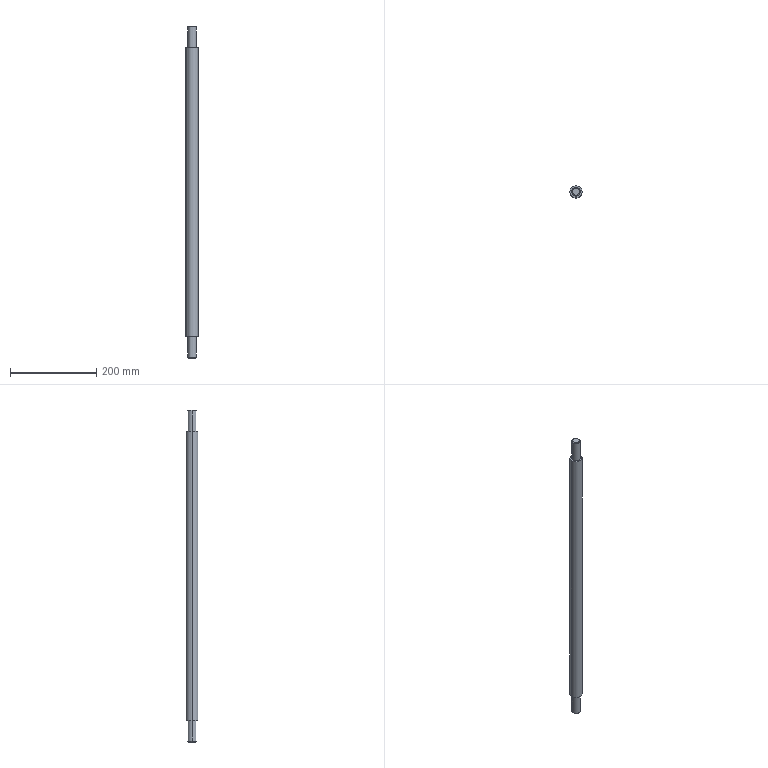Part | Creo | features DATUM PLANE 3, CURVE 2, PROTRUSION 2, CHAMFER 1, COORDINATE SYSTEM 1 | 1 solid | 14 faces | box 28 x 28 x 770 mm | volume 443735 mm3 | cylinder 6 | plane 4 | cone 4 | commonest cylinder face diameters 20 x4 28 x2
STEP:
#1=CARTESIAN_POINT('',(0.,0.,0.));
#2=DIRECTION('',(0.,0.,1.));
#3=DIRECTION('',(1.,0.,0.));
#4=AXIS2_PLACEMENT_3D('',#1,#2,#3);
#5=CARTESIAN_POINT('',(14.,0.,-335.));
#6=VERTEX_POINT('',#5);
#7=CARTESIAN_POINT('',(-14.,0.,-335.));
#8=VERTEX_POINT('',#7);
#9=CARTESIAN_POINT('',(0.,0.,-335.));
#10=DIRECTION('',(0.,0.,1.));
#11=DIRECTION('',(1.,0.,0.));
#12=AXIS2_PLACEMENT_3D('',#9,#10,#11);
#13=CIRCLE('',#12,14.);
#14=EDGE_CURVE('',#6,#8,#13,.T.);
#15=ORIENTED_EDGE('',*,*,#14,.T.);
#16=CARTESIAN_POINT('',(0.,0.,-335.));
#17=DIRECTION('',(0.,0.,1.));
#18=DIRECTION('',(-1.,0.,0.));
#19=AXIS2_PLACEMENT_3D('',#16,#17,#18);
#20=CIRCLE('',#19,14.);
#21=EDGE_CURVE('',#8,#6,#20,.T.);
#22=ORIENTED_EDGE('',*,*,#21,.T.);
#23=EDGE_LOOP('',(#15,#22));
#24=FACE_OUTER_BOUND('',#23,.F.);
#25=CARTESIAN_POINT('',(10.,0.,-335.));
#26=VERTEX_POINT('',#25);
#27=CARTESIAN_POINT('',(-10.,0.,-335.));
#28=VERTEX_POINT('',#27);
#29=CARTESIAN_POINT('',(0.,0.,-335.));
#30=DIRECTION('',(0.,0.,1.));
#31=DIRECTION('',(1.,0.,0.));
#32=AXIS2_PLACEMENT_3D('',#29,#30,#31);
#33=CIRCLE('',#32,10.);
#34=EDGE_CURVE('',#26,#28,#33,.T.);
#35=ORIENTED_EDGE('',*,*,#34,.F.);
#36=CARTESIAN_POINT('',(0.,0.,-335.));
#37=DIRECTION('',(0.,0.,1.));
#38=DIRECTION('',(-1.,0.,0.));
#39=AXIS2_PLACEMENT_3D('',#36,#37,#38);
#40=CIRCLE('',#39,10.);
#41=EDGE_CURVE('',#28,#26,#40,.T.);
#42=ORIENTED_EDGE('',*,*,#41,.F.);
#43=EDGE_LOOP('',(#35,#42));
#44=FACE_BOUND('',#43,.F.);
#45=CARTESIAN_POINT('',(0.,0.,-335.));
#46=DIRECTION('',(0.,0.,1.));
#47=DIRECTION('',(1.,0.,0.));
#48=AXIS2_PLACEMENT_3D('',#45,#46,#47);
#49=PLANE('',#48);
#50=ADVANCED_FACE('',(#24,#44),#49,.F.);
#51=ORIENTED_EDGE('',*,*,#14,.F.);
#52=CARTESIAN_POINT('',(14.,0.,335.));
#53=VERTEX_POINT('',#52);
#54=CARTESIAN_POINT('',(14.,0.,-335.));
#55=DIRECTION('',(0.,0.,1.));
#56=VECTOR('',#55,670.);
#57=LINE('',#54,#56);
#58=EDGE_CURVE('',#6,#53,#57,.T.);
#59=ORIENTED_EDGE('',*,*,#58,.T.);
#60=CARTESIAN_POINT('',(-14.,0.,335.));
#61=VERTEX_POINT('',#60);
#62=CARTESIAN_POINT('',(0.,0.,335.));
#63=DIRECTION('',(0.,0.,1.));
#64=DIRECTION('',(1.,0.,0.));
#65=AXIS2_PLACEMENT_3D('',#62,#63,#64);
#66=CIRCLE('',#65,14.);
#67=EDGE_CURVE('',#53,#61,#66,.T.);
#68=ORIENTED_EDGE('',*,*,#67,.T.);
#69=CARTESIAN_POINT('',(-14.,0.,-335.));
#70=DIRECTION('',(0.,0.,1.));
#71=VECTOR('',#70,670.);
#72=LINE('',#69,#71);
#73=EDGE_CURVE('',#8,#61,#72,.T.);
#74=ORIENTED_EDGE('',*,*,#73,.F.);
#75=EDGE_LOOP('',(#51,#59,#68,#74));
#76=FACE_OUTER_BOUND('',#75,.F.);
#77=CARTESIAN_POINT('',(0.,0.,-335.));
#78=DIRECTION('',(0.,0.,1.));
#79=DIRECTION('',(1.,0.,0.));
#80=AXIS2_PLACEMENT_3D('',#77,#78,#79);
#81=CYLINDRICAL_SURFACE('',#80,14.);
#82=ADVANCED_FACE('',(#76),#81,.T.);
#83=ORIENTED_EDGE('',*,*,#21,.F.);
#84=ORIENTED_EDGE('',*,*,#73,.T.);
#85=CARTESIAN_POINT('',(0.,0.,335.));
#86=DIRECTION('',(0.,0.,1.));
#87=DIRECTION('',(-1.,0.,0.));
#88=AXIS2_PLACEMENT_3D('',#85,#86,#87);
#89=CIRCLE('',#88,14.);
#90=EDGE_CURVE('',#61,#53,#89,.T.);
#91=ORIENTED_EDGE('',*,*,#90,.T.);
#92=ORIENTED_EDGE('',*,*,#58,.F.);
#93=EDGE_LOOP('',(#83,#84,#91,#92));
#94=FACE_OUTER_BOUND('',#93,.F.);
#95=CARTESIAN_POINT('',(0.,0.,-335.));
#96=DIRECTION('',(0.,0.,1.));
#97=DIRECTION('',(1.,0.,0.));
#98=AXIS2_PLACEMENT_3D('',#95,#96,#97);
#99=CYLINDRICAL_SURFACE('',#98,14.);
#100=ADVANCED_FACE('',(#94),#99,.T.);
#101=ORIENTED_EDGE('',*,*,#67,.F.);
#102=ORIENTED_EDGE('',*,*,#90,.F.);
#103=EDGE_LOOP('',(#101,#102));
#104=FACE_OUTER_BOUND('',#103,.F.);
#105=CARTESIAN_POINT('',(10.,0.,335.));
#106=VERTEX_POINT('',#105);
#107=CARTESIAN_POINT('',(-10.,0.,335.));
#108=VERTEX_POINT('',#107);
#109=CARTESIAN_POINT('',(0.,0.,335.));
#110=DIRECTION('',(0.,0.,1.));
#111=DIRECTION('',(1.,0.,0.));
#112=AXIS2_PLACEMENT_3D('',#109,#110,#111);
#113=CIRCLE('',#112,10.);
#114=EDGE_CURVE('',#106,#108,#113,.T.);
#115=ORIENTED_EDGE('',*,*,#114,.T.);
#116=CARTESIAN_POINT('',(0.,0.,335.));
#117=DIRECTION('',(0.,0.,1.));
#118=DIRECTION('',(-1.,0.,0.));
#119=AXIS2_PLACEMENT_3D('',#116,#117,#118);
#120=CIRCLE('',#119,10.);
#121=EDGE_CURVE('',#108,#106,#120,.T.);
#122=ORIENTED_EDGE('',*,*,#121,.T.);
#123=EDGE_LOOP('',(#115,#122));
#124=FACE_BOUND('',#123,.F.);
#125=CARTESIAN_POINT('',(0.,0.,335.));
#126=DIRECTION('',(0.,0.,1.));
#127=DIRECTION('',(1.,0.,0.));
#128=AXIS2_PLACEMENT_3D('',#125,#126,#127);
#129=PLANE('',#128);
#130=ADVANCED_FACE('',(#104,#124),#129,.T.);
#131=CARTESIAN_POINT('',(10.,0.,383.));
#132=VERTEX_POINT('',#131);
#133=CARTESIAN_POINT('',(-10.,0.,383.));
#134=VERTEX_POINT('',#133);
#135=CARTESIAN_POINT('',(0.,0.,383.));
#136=DIRECTION('',(0.,0.,1.));
#137=DIRECTION('',(1.,0.,0.));
#138=AXIS2_PLACEMENT_3D('',#135,#136,#137);
#139=CIRCLE('',#138,10.);
#140=EDGE_CURVE('',#132,#134,#139,.T.);
#141=ORIENTED_EDGE('',*,*,#140,.T.);
#142=CARTESIAN_POINT('',(-10.,0.,335.));
#143=DIRECTION('',(0.000000001,-0.000000003,1.));
#144=VECTOR('',#143,48.);
#145=LINE('',#142,#144);
#146=EDGE_CURVE('',#108,#134,#145,.T.);
#147=ORIENTED_EDGE('',*,*,#146,.F.);
#148=ORIENTED_EDGE('',*,*,#114,.F.);
#149=CARTESIAN_POINT('',(10.,0.,335.));
#150=DIRECTION('',(-0.000000001,0.000000003,1.));
#151=VECTOR('',#150,48.);
#152=LINE('',#149,#151);
#153=EDGE_CURVE('',#106,#132,#152,.T.);
#154=ORIENTED_EDGE('',*,*,#153,.T.);
#155=EDGE_LOOP('',(#141,#147,#148,#154));
#156=FACE_OUTER_BOUND('',#155,.F.);
#157=CARTESIAN_POINT('',(0.,0.,-385.));
#158=DIRECTION('',(0.,0.,1.));
#159=DIRECTION('',(1.,0.,0.));
#160=AXIS2_PLACEMENT_3D('',#157,#158,#159);
#161=CYLINDRICAL_SURFACE('',#160,10.);
#162=ADVANCED_FACE('',(#156),#161,.T.);
#163=CARTESIAN_POINT('',(-10.,0.,-383.));
#164=VERTEX_POINT('',#163);
#165=CARTESIAN_POINT('',(10.,0.,-383.));
#166=VERTEX_POINT('',#165);
#167=CARTESIAN_POINT('',(0.,0.,-383.));
#168=DIRECTION('',(0.,0.,-1.));
#169=DIRECTION('',(-1.,0.,0.));
#170=AXIS2_PLACEMENT_3D('',#167,#168,#169);
#171=CIRCLE('',#170,10.);
#172=EDGE_CURVE('',#164,#166,#171,.T.);
#173=ORIENTED_EDGE('',*,*,#172,.T.);
#174=CARTESIAN_POINT('',(10.,0.000000146,-383.));
#175=DIRECTION('',(0.000000001,-0.000000003,1.));
#176=VECTOR('',#175,48.);
#177=LINE('',#174,#176);
#178=EDGE_CURVE('',#166,#26,#177,.T.);
#179=ORIENTED_EDGE('',*,*,#178,.T.);
#180=ORIENTED_EDGE('',*,*,#34,.T.);
#181=CARTESIAN_POINT('',(-10.,-0.000000146,-383.));
#182=DIRECTION('',(-0.000000001,0.000000003,1.));
#183=VECTOR('',#182,48.);
#184=LINE('',#181,#183);
#185=EDGE_CURVE('',#164,#28,#184,.T.);
#186=ORIENTED_EDGE('',*,*,#185,.F.);
#187=EDGE_LOOP('',(#173,#179,#180,#186));
#188=FACE_OUTER_BOUND('',#187,.F.);
#189=CARTESIAN_POINT('',(0.,0.,-385.));
#190=DIRECTION('',(0.,0.,1.));
#191=DIRECTION('',(1.,0.,0.));
#192=AXIS2_PLACEMENT_3D('',#189,#190,#191);
#193=CYLINDRICAL_SURFACE('',#192,10.);
#194=ADVANCED_FACE('',(#188),#193,.T.);
#195=CARTESIAN_POINT('',(8.,0.,385.));
#196=VERTEX_POINT('',#195);
#197=CARTESIAN_POINT('',(-8.,0.,385.));
#198=VERTEX_POINT('',#197);
#199=CARTESIAN_POINT('',(0.,0.,385.));
#200=DIRECTION('',(0.,0.,1.));
#201=DIRECTION('',(1.,0.,0.));
#202=AXIS2_PLACEMENT_3D('',#199,#200,#201);
#203=CIRCLE('',#202,8.);
#204=EDGE_CURVE('',#196,#198,#203,.T.);
#205=ORIENTED_EDGE('',*,*,#204,.T.);
#206=CARTESIAN_POINT('',(-8.,-0.000000156,385.));
#207=DIRECTION('',(-0.7071,0.000000003,-0.7071));
#208=VECTOR('',#207,2.828);
#209=LINE('',#206,#208);
#210=EDGE_CURVE('',#198,#134,#209,.T.);
#211=ORIENTED_EDGE('',*,*,#210,.T.);
#212=ORIENTED_EDGE('',*,*,#140,.F.);
#213=CARTESIAN_POINT('',(8.,0.000000156,385.));
#214=DIRECTION('',(0.7071,-0.000000003,-0.7071));
#215=VECTOR('',#214,2.828);
#216=LINE('',#213,#215);
#217=EDGE_CURVE('',#196,#132,#216,.T.);
#218=ORIENTED_EDGE('',*,*,#217,.F.);
#219=EDGE_LOOP('',(#205,#211,#212,#218));
#220=FACE_OUTER_BOUND('',#219,.F.);
#221=CARTESIAN_POINT('',(0.,0.,384.));
#222=DIRECTION('',(0.,0.,-1.));
#223=DIRECTION('',(0.,-1.,0.));
#224=AXIS2_PLACEMENT_3D('',#221,#222,#223);
#225=CONICAL_SURFACE('',#224,9.,45.);
#226=ADVANCED_FACE('',(#220),#225,.T.);
#227=CARTESIAN_POINT('',(0.,0.,385.));
#228=DIRECTION('',(0.,0.,1.));
#229=DIRECTION('',(-1.,0.,0.));
#230=AXIS2_PLACEMENT_3D('',#227,#228,#229);
#231=CIRCLE('',#230,8.);
#232=EDGE_CURVE('',#198,#196,#231,.T.);
#233=ORIENTED_EDGE('',*,*,#232,.F.);
#234=ORIENTED_EDGE('',*,*,#204,.F.);
#235=EDGE_LOOP('',(#233,#234));
#236=FACE_OUTER_BOUND('',#235,.F.);
#237=CARTESIAN_POINT('',(0.,0.,385.));
#238=DIRECTION('',(0.,0.,1.));
#239=DIRECTION('',(1.,0.,0.));
#240=AXIS2_PLACEMENT_3D('',#237,#238,#239);
#241=PLANE('',#240);
#242=ADVANCED_FACE('',(#236),#241,.T.);
#243=ORIENTED_EDGE('',*,*,#232,.T.);
#244=ORIENTED_EDGE('',*,*,#217,.T.);
#245=CARTESIAN_POINT('',(0.,0.,383.));
#246=DIRECTION('',(0.,0.,1.));
#247=DIRECTION('',(-1.,0.,0.));
#248=AXIS2_PLACEMENT_3D('',#245,#246,#247);
#249=CIRCLE('',#248,10.);
#250=EDGE_CURVE('',#134,#132,#249,.T.);
#251=ORIENTED_EDGE('',*,*,#250,.F.);
#252=ORIENTED_EDGE('',*,*,#210,.F.);
#253=EDGE_LOOP('',(#243,#244,#251,#252));
#254=FACE_OUTER_BOUND('',#253,.F.);
#255=CARTESIAN_POINT('',(0.,0.,384.));
#256=DIRECTION('',(0.,0.,-1.));
#257=DIRECTION('',(0.,-1.,0.));
#258=AXIS2_PLACEMENT_3D('',#255,#256,#257);
#259=CONICAL_SURFACE('',#258,9.,45.);
#260=ADVANCED_FACE('',(#254),#259,.T.);
#261=ORIENTED_EDGE('',*,*,#250,.T.);
#262=ORIENTED_EDGE('',*,*,#153,.F.);
#263=ORIENTED_EDGE('',*,*,#121,.F.);
#264=ORIENTED_EDGE('',*,*,#146,.T.);
#265=EDGE_LOOP('',(#261,#262,#263,#264));
#266=FACE_OUTER_BOUND('',#265,.F.);
#267=CARTESIAN_POINT('',(0.,0.,-385.));
#268=DIRECTION('',(0.,0.,1.));
#269=DIRECTION('',(1.,0.,0.));
#270=AXIS2_PLACEMENT_3D('',#267,#268,#269);
#271=CYLINDRICAL_SURFACE('',#270,10.);
#272=ADVANCED_FACE('',(#266),#271,.T.);
#273=CARTESIAN_POINT('',(0.,0.,-383.));
#274=DIRECTION('',(0.,0.,-1.));
#275=DIRECTION('',(1.,0.,0.));
#276=AXIS2_PLACEMENT_3D('',#273,#274,#275);
#277=CIRCLE('',#276,10.);
#278=EDGE_CURVE('',#166,#164,#277,.T.);
#279=ORIENTED_EDGE('',*,*,#278,.T.);
#280=ORIENTED_EDGE('',*,*,#185,.T.);
#281=ORIENTED_EDGE('',*,*,#41,.T.);
#282=ORIENTED_EDGE('',*,*,#178,.F.);
#283=EDGE_LOOP('',(#279,#280,#281,#282));
#284=FACE_OUTER_BOUND('',#283,.F.);
#285=CARTESIAN_POINT('',(0.,0.,-385.));
#286=DIRECTION('',(0.,0.,1.));
#287=DIRECTION('',(1.,0.,0.));
#288=AXIS2_PLACEMENT_3D('',#285,#286,#287);
#289=CYLINDRICAL_SURFACE('',#288,10.);
#290=ADVANCED_FACE('',(#284),#289,.T.);
#291=CARTESIAN_POINT('',(8.,0.,-385.));
#292=VERTEX_POINT('',#291);
#293=CARTESIAN_POINT('',(-8.,0.,-385.));
#294=VERTEX_POINT('',#293);
#295=CARTESIAN_POINT('',(0.,0.,-385.));
#296=DIRECTION('',(0.,0.,-1.));
#297=DIRECTION('',(1.,0.,0.));
#298=AXIS2_PLACEMENT_3D('',#295,#296,#297);
#299=CIRCLE('',#298,8.);
#300=EDGE_CURVE('',#292,#294,#299,.T.);
#301=ORIENTED_EDGE('',*,*,#300,.T.);
#302=CARTESIAN_POINT('',(-8.,-0.000000156,-385.));
#303=DIRECTION('',(-0.7071,0.000000003,0.7071));
#304=VECTOR('',#303,2.828);
#305=LINE('',#302,#304);
#306=EDGE_CURVE('',#294,#164,#305,.T.);
#307=ORIENTED_EDGE('',*,*,#306,.T.);
#308=ORIENTED_EDGE('',*,*,#278,.F.);
#309=CARTESIAN_POINT('',(8.,0.000000156,-385.));
#310=DIRECTION('',(0.7071,-0.000000003,0.7071));
#311=VECTOR('',#310,2.828);
#312=LINE('',#309,#311);
#313=EDGE_CURVE('',#292,#166,#312,.T.);
#314=ORIENTED_EDGE('',*,*,#313,.F.);
#315=EDGE_LOOP('',(#301,#307,#308,#314));
#316=FACE_OUTER_BOUND('',#315,.F.);
#317=CARTESIAN_POINT('',(0.,0.,-384.));
#318=DIRECTION('',(0.,0.,1.));
#319=DIRECTION('',(0.,-1.,0.));
#320=AXIS2_PLACEMENT_3D('',#317,#318,#319);
#321=CONICAL_SURFACE('',#320,9.,45.);
#322=ADVANCED_FACE('',(#316),#321,.T.);
#323=ORIENTED_EDGE('',*,*,#300,.F.);
#324=CARTESIAN_POINT('',(0.,0.,-385.));
#325=DIRECTION('',(0.,0.,-1.));
#326=DIRECTION('',(-1.,0.,0.));
#327=AXIS2_PLACEMENT_3D('',#324,#325,#326);
#328=CIRCLE('',#327,8.);
#329=EDGE_CURVE('',#294,#292,#328,.T.);
#330=ORIENTED_EDGE('',*,*,#329,.F.);
#331=EDGE_LOOP('',(#323,#330));
#332=FACE_OUTER_BOUND('',#331,.F.);
#333=CARTESIAN_POINT('',(0.,0.,-385.));
#334=DIRECTION('',(0.,0.,1.));
#335=DIRECTION('',(1.,0.,0.));
#336=AXIS2_PLACEMENT_3D('',#333,#334,#335);
#337=PLANE('',#336);
#338=ADVANCED_FACE('',(#332),#337,.F.);
#339=ORIENTED_EDGE('',*,*,#329,.T.);
#340=ORIENTED_EDGE('',*,*,#313,.T.);
#341=ORIENTED_EDGE('',*,*,#172,.F.);
#342=ORIENTED_EDGE('',*,*,#306,.F.);
#343=EDGE_LOOP('',(#339,#340,#341,#342));
#344=FACE_OUTER_BOUND('',#343,.F.);
#345=CARTESIAN_POINT('',(0.,0.,-384.));
#346=DIRECTION('',(0.,0.,1.));
#347=DIRECTION('',(0.,-1.,0.));
#348=AXIS2_PLACEMENT_3D('',#345,#346,#347);
#349=CONICAL_SURFACE('',#348,9.,45.);
#350=ADVANCED_FACE('',(#344),#349,.T.);
#351=CLOSED_SHELL('',(#50,#82,#100,#130,#162,#194,#226,#242,#260,#272,#290,#322,#338,#350));
#352=MANIFOLD_SOLID_BREP('',#351);
#353=(LENGTH_UNIT()NAMED_UNIT(*)SI_UNIT(.MILLI.,.METRE.));
#354=UNCERTAINTY_MEASURE_WITH_UNIT(LENGTH_MEASURE(0.0771),#353,'','');
#355=(NAMED_UNIT(*)PLANE_ANGLE_UNIT()SI_UNIT($,.RADIAN.));
#356=PLANE_ANGLE_MEASURE_WITH_UNIT(PLANE_ANGLE_MEASURE(0.01745),#355);
#357=(CONVERSION_BASED_UNIT('DEGREE',#356)NAMED_UNIT(*)PLANE_ANGLE_UNIT());
#358=(NAMED_UNIT(*)SI_UNIT($,.STERADIAN.)SOLID_ANGLE_UNIT());
#359=(GEOMETRIC_REPRESENTATION_CONTEXT(3)GLOBAL_UNCERTAINTY_ASSIGNED_CONTEXT((#354))GLOBAL_UNIT_ASSIGNED_CONTEXT((#353,#357,#358))REPRESENTATION_CONTEXT('',''));
#360=ADVANCED_BREP_SHAPE_REPRESENTATION('',(#4,#352),#359);